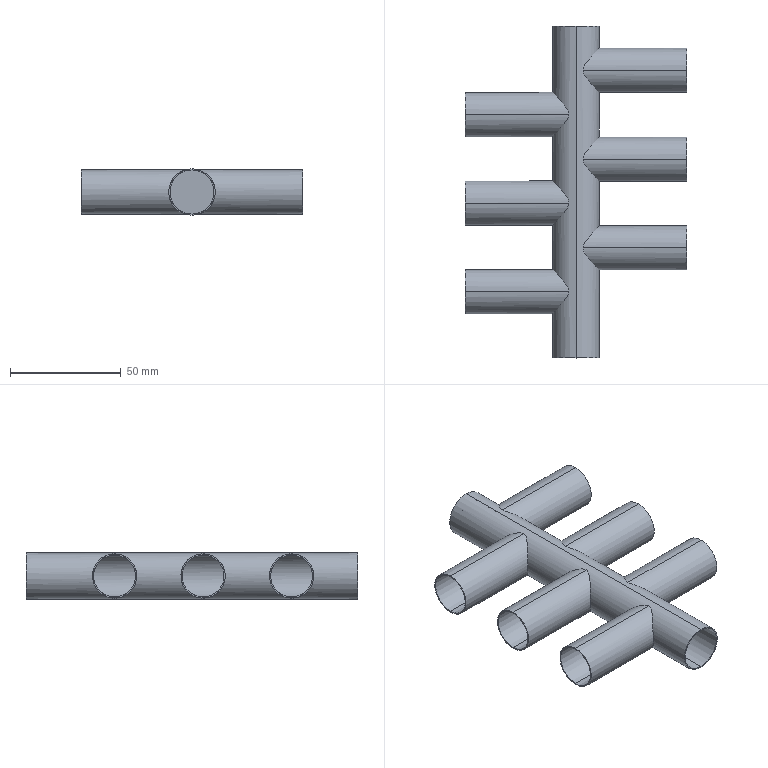Part | SolidWorks | features ICE 5, Extrusion 1 | 1 solid | 43 faces | box 100 x 150 x 21 mm | volume 13196 mm3 | cylinder 28 | plane 15 | commonest cylinder face diameters 20 x14 19 x12 21 x2